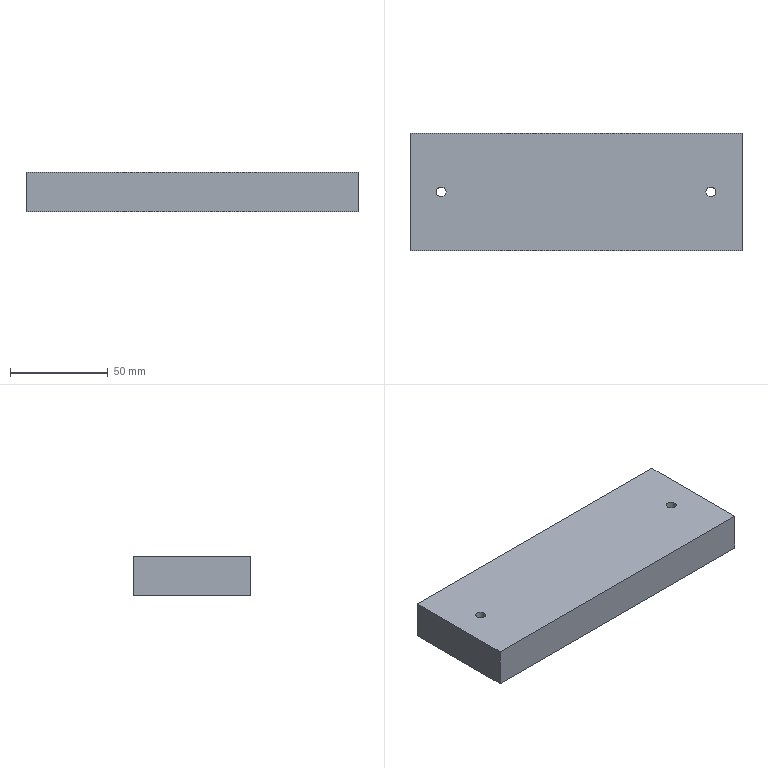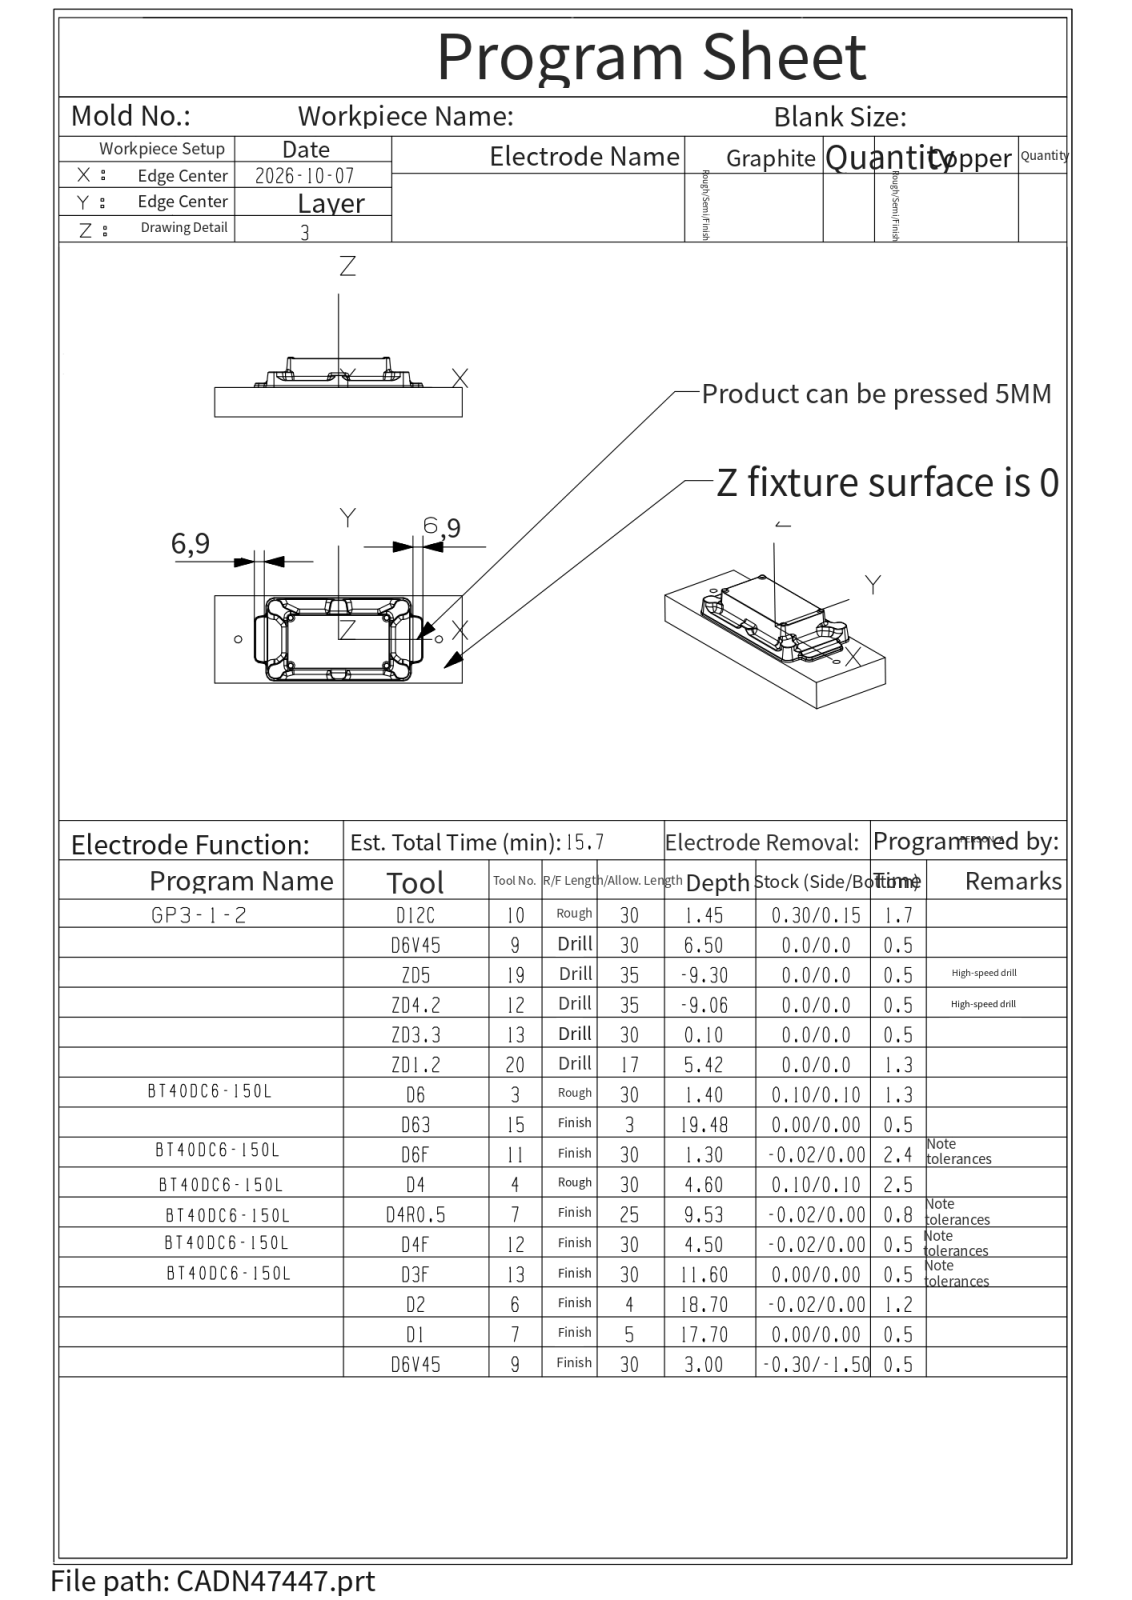NC program | NX | posted by the shop | part box 170 x 60 x 20 mm
Lines 6151 to 7072 of 17682:
T05 M06
T20
( name=D3    T=5 )
( XY = 0.10 )
( Z = 0.10 )
G00 G90 G54 X-19.944 Y-32.3 S10000 M03
G43 Z27.98 H05 M08
Z17.38
G03 X-19.344 Y-32.9 I.6 J0.0 F1600.
G01 X-18.41 F2000.
G03 X-18. Y-32.5 I.01 J.4
G01 Y-31.556
G03 X-18.6 Y-30.956 I-.6 J0.0
G01 X-19.944 Y-32.3 Z17.18 F6000.
G03 X-19.344 Y-32.9 I.6 J0.0 F1600.
G01 X-18.4 F2000.
G03 X-18. Y-32.5 I0.0 J.4
G01 Y-31.556
G03 X-18.6 Y-30.956 I-.6 J0.0
G01 X-19.944 Y-32.3 Z16.98 F6000.
G03 X-19.344 Y-32.9 I.6 J0.0 F1600.
G01 X-18.4 F2000.
G03 X-18. Y-32.5 I0.0 J.4
G01 Y-31.556
G03 X-18.6 Y-30.956 I-.6 J0.0
G01 X-19.944 Y-32.3 Z16.78 F6000.
G03 X-19.344 Y-32.9 I.6 J0.0 F1600.
G01 X-18.4 F2000.
G03 X-18. Y-32.5 I0.0 J.4
G01 Y-31.556
G03 X-18.6 Y-30.956 I-.6 J0.0
G01 X-19.944 Y-32.3 Z16.58 F6000.
G03 X-19.344 Y-32.9 I.6 J0.0 F1600.
G01 X-18.4 F2000.
G03 X-18. Y-32.5 I0.0 J.4
G01 Y-31.556
G03 X-18.6 Y-30.956 I-.6 J0.0
G01 X-19.944 Y-32.3 Z16.38 F6000.
G03 X-19.344 Y-32.9 I.6 J0.0 F1600.
G01 X-18.4 F2000.
G03 X-18. Y-32.5 I0.0 J.4
G01 Y-31.556
G03 X-18.6 Y-30.956 I-.6 J0.0
G01 X-19.944 Y-32.3 Z16.18 F6000.
G03 X-19.344 Y-32.9 I.6 J0.0 F1600.
G01 X-18.4 F2000.
G03 X-18. Y-32.5 I0.0 J.4
G01 Y-31.556
G03 X-18.6 Y-30.956 I-.6 J0.0
G01 X-19.944 Y-32.3 Z15.98 F6000.
G03 X-19.344 Y-32.9 I.6 J0.0 F1600.
G01 X-18.4 F2000.
G03 X-18. Y-32.5 I0.0 J.4
G01 Y-31.556
G03 X-18.6 Y-30.956 I-.6 J0.0
G01 X-19.944 Y-32.3 Z15.78 F6000.
G03 X-19.344 Y-32.9 I.6 J0.0 F1600.
G01 X-18.4 F2000.
G03 X-18. Y-32.5 I0.0 J.4
G01 Y-31.556
G03 X-18.6 Y-30.956 I-.6 J0.0
G01 X-19.944 Y-32.3 Z15.58 F6000.
G03 X-19.344 Y-32.9 I.6 J0.0 F1600.
G01 X-18.4 F2000.
G03 X-18. Y-32.5 I0.0 J.4
G01 Y-31.556
G03 X-18.6 Y-30.956 I-.6 J0.0
G01 X-19.944 Y-32.3 Z15.38 F6000.
G03 X-19.344 Y-32.9 I.6 J0.0 F1600.
G01 X-18.4 F2000.
G03 X-18. Y-32.5 I0.0 J.4
G01 Y-31.556
G03 X-18.6 Y-30.956 I-.6 J0.0
G01 X-19.944 Y-32.3 Z15.18 F6000.
G03 X-19.344 Y-32.9 I.6 J0.0 F1600.
G01 X-18.4 F2000.
G03 X-18. Y-32.5 I0.0 J.4
G01 Y-31.556
G03 X-18.6 Y-30.956 I-.6 J0.0
G01 X-19.944 Y-32.3 Z14.98 F6000.
G03 X-19.344 Y-32.9 I.6 J0.0 F1600.
G01 X-18.4 F2000.
G03 X-18. Y-32.5 I0.0 J.4
G01 Y-31.556
G03 X-18.6 Y-30.956 I-.6 J0.0
G01 X-19.944 Y-32.3 Z14.78 F6000.
G03 X-19.344 Y-32.9 I.6 J0.0 F1600.
G01 X-18.4 F2000.
G03 X-18. Y-32.5 I0.0 J.4
G01 Y-31.556
G03 X-18.6 Y-30.956 I-.6 J0.0
G01 X-19.944 Y-32.3 Z14.58 F6000.
G03 X-19.344 Y-32.9 I.6 J0.0 F1600.
G01 X-18.4 F2000.
G03 X-18. Y-32.5 I0.0 J.4
G01 Y-31.556
G03 X-18.6 Y-30.956 I-.6 J0.0
G01 X-19.944 Y-32.3 Z14.38 F6000.
G03 X-19.344 Y-32.9 I.6 J0.0 F1600.
G01 X-18.4 F2000.
G03 X-18. Y-32.5 I0.0 J.4
G01 Y-31.556
G03 X-18.6 Y-30.956 I-.6 J0.0
G01 X-19.944 Y-32.3 Z14.18 F6000.
G03 X-19.344 Y-32.9 I.6 J0.0 F1600.
G01 X-18.4 F2000.
G03 X-18. Y-32.5 I0.0 J.4
G01 Y-31.556
G03 X-18.6 Y-30.956 I-.6 J0.0
G01 X-19.944 Y-32.3 Z13.98 F6000.
G03 X-19.344 Y-32.9 I.6 J0.0 F1600.
G01 X-18.4 F2000.
G03 X-18. Y-32.5 I0.0 J.4
G01 Y-31.556
G03 X-18.6 Y-30.956 I-.6 J0.0
G01 X-19.944 Y-32.3 Z13.78 F6000.
G03 X-19.344 Y-32.9 I.6 J0.0 F1600.
G01 X-18.4 F2000.
G03 X-18. Y-32.5 I0.0 J.4
G01 Y-31.556
G03 X-18.6 Y-30.956 I-.6 J0.0
G01 X-19.944 Y-32.3 Z13.58 F6000.
G03 X-19.344 Y-32.9 I.6 J0.0 F1600.
G01 X-18.4 F2000.
G03 X-18. Y-32.5 I0.0 J.4
G01 Y-31.556
G03 X-18.6 Y-30.956 I-.6 J0.0
G01 X-19.944 Y-32.3 Z13.38 F6000.
G03 X-19.344 Y-32.9 I.6 J0.0 F1600.
G01 X-18.4 F2000.
G03 X-18. Y-32.5 I0.0 J.4
G01 Y-31.556
G03 X-18.6 Y-30.956 I-.6 J0.0
G01 X-19.944 Y-32.3 Z13.18 F6000.
G03 X-19.344 Y-32.9 I.6 J0.0 F1600.
G01 X-18.4 F2000.
G03 X-18. Y-32.5 I0.0 J.4
G01 Y-31.556
G03 X-18.6 Y-30.956 I-.6 J0.0
G01 X-19.944 Y-32.3 Z12.98 F6000.
G03 X-19.344 Y-32.9 I.6 J0.0 F1600.
G01 X-18.4 F2000.
G03 X-18. Y-32.5 I0.0 J.4
G01 Y-31.556
G03 X-18.6 Y-30.956 I-.6 J0.0
G01 X-19.944 Y-32.3 Z12.78 F6000.
G03 X-19.344 Y-32.9 I.6 J0.0 F1600.
G01 X-18.4 F2000.
G03 X-18. Y-32.5 I0.0 J.4
G01 Y-31.556
G03 X-18.6 Y-30.956 I-.6 J0.0
G01 X-19.944 Y-32.3 Z12.58 F6000.
G03 X-19.344 Y-32.9 I.6 J0.0 F1600.
G01 X-18.4 F2000.
G03 X-18. Y-32.5 I0.0 J.4
G01 Y-31.556
G03 X-18.6 Y-30.956 I-.6 J0.0
G01 X-19.944 Y-32.3 Z12.38 F6000.
G03 X-19.344 Y-32.9 I.6 J0.0 F1600.
G01 X-18.4 F2000.
G03 X-18. Y-32.5 I0.0 J.4
G01 Y-31.556
G03 X-18.6 Y-30.956 I-.6 J0.0
G01 X-19.944 Y-32.3 Z12.18 F6000.
G03 X-19.344 Y-32.9 I.6 J0.0 F1600.
G01 X-18.4 F2000.
G03 X-18. Y-32.5 I0.0 J.4
G01 Y-31.556
G03 X-18.6 Y-30.956 I-.6 J0.0
G01 X-19.944 Y-32.3 Z11.98 F6000.
G03 X-19.344 Y-32.9 I.6 J0.0 F1600.
G01 X-18.4 F2000.
G03 X-18. Y-32.5 I0.0 J.4
G01 Y-31.556
G03 X-18.6 Y-30.956 I-.6 J0.0
G01 X-19.944 Y-32.3 Z11.78 F6000.
G03 X-19.344 Y-32.9 I.6 J0.0 F1600.
G01 X-18.4 F2000.
G03 X-18. Y-32.5 I0.0 J.4
G01 Y-31.556
G03 X-18.6 Y-30.956 I-.6 J0.0
G01 X-19.944 Y-32.3 Z11.58 F6000.
G03 X-19.344 Y-32.9 I.6 J0.0 F1600.
G01 X-18.4 F2000.
G03 X-18. Y-32.5 I0.0 J.4
G01 Y-31.556
G03 X-18.6 Y-30.956 I-.6 J0.0
G01 X-19.944 Y-32.3 Z11.38 F6000.
G03 X-19.344 Y-32.9 I.6 J0.0 F1600.
G01 X-18.4 F2000.
G03 X-18. Y-32.5 I0.0 J.4
G01 Y-31.556
G03 X-18.6 Y-30.956 I-.6 J0.0
G01 X-19.944 Y-32.3 Z11.18 F6000.
G03 X-19.344 Y-32.9 I.6 J0.0 F1600.
G01 X-18.4 F2000.
G03 X-18. Y-32.5 I0.0 J.4
G01 Y-31.556
G03 X-18.6 Y-30.956 I-.6 J0.0
G01 X-19.944 Y-32.3 Z10.98 F6000.
G03 X-19.344 Y-32.9 I.6 J0.0 F1600.
G01 X-18.4 F2000.
G03 X-18. Y-32.5 I0.0 J.4
G01 Y-31.556
G03 X-18.6 Y-30.956 I-.6 J0.0
G01 X-19.944 Y-32.3 Z10.78 F6000.
G03 X-19.344 Y-32.9 I.6 J0.0 F1600.
G01 X-18.4 F2000.
G03 X-18. Y-32.5 I0.0 J.4
G01 Y-31.556
G03 X-18.6 Y-30.956 I-.6 J0.0
G01 X-19.944 Y-32.3 Z10.58 F6000.
G03 X-19.344 Y-32.9 I.6 J0.0 F1600.
G01 X-18.4 F2000.
G03 X-18. Y-32.5 I0.0 J.4
G01 Y-31.556
G03 X-18.6 Y-30.956 I-.6 J0.0
G01 X-19.944 Y-32.3 Z10.38 F6000.
G03 X-19.344 Y-32.9 I.6 J0.0 F1600.
G01 X-18.4 F2000.
G03 X-18. Y-32.5 I0.0 J.4
G01 Y-31.556
G03 X-18.6 Y-30.956 I-.6 J0.0
G01 X-19.944 Y-32.3 Z10.18 F6000.
G03 X-19.344 Y-32.9 I.6 J0.0 F1600.
G01 X-18.4 F2000.
G03 X-18. Y-32.5 I0.0 J.4
G01 Y-31.556
G03 X-18.6 Y-30.956 I-.6 J0.0
G01 X-19.944 Y-32.3 Z9.98 F6000.
G03 X-19.344 Y-32.9 I.6 J0.0 F1600.
G01 X-18.4 F2000.
G03 X-18. Y-32.5 I0.0 J.4
G01 Y-31.556
G03 X-18.6 Y-30.956 I-.6 J0.0
G01 X-19.944 Y-32.3 Z9.78 F6000.
G03 X-19.344 Y-32.9 I.6 J0.0 F1600.
G01 X-18.4 F2000.
G03 X-18. Y-32.5 I0.0 J.4
G01 Y-31.556
G03 X-18.6 Y-30.956 I-.6 J0.0
G01 X-19.944 Y-32.3 Z9.58 F6000.
G03 X-19.344 Y-32.9 I.6 J0.0 F1600.
G01 X-18.4 F2000.
G03 X-18. Y-32.5 I0.0 J.4
G01 Y-31.556
G03 X-18.6 Y-30.956 I-.6 J0.0
G01 X-19.944 Y-32.3 Z9.38 F6000.
G03 X-19.344 Y-32.9 I.6 J0.0 F1600.
G01 X-18.4 F2000.
G03 X-18. Y-32.5 I0.0 J.4
G01 Y-31.556
G03 X-18.6 Y-30.956 I-.6 J0.0
G01 X-19.944 Y-32.3 Z9.18 F6000.
G03 X-19.344 Y-32.9 I.6 J0.0 F1600.
G01 X-18.4 F2000.
G03 X-18. Y-32.5 I0.0 J.4
G01 Y-31.556
G03 X-18.6 Y-30.956 I-.6 J0.0
G01 X-19.944 Y-32.3 Z8.98 F6000.
G03 X-19.344 Y-32.9 I.6 J0.0 F1600.
G01 X-18.4 F2000.
G03 X-18. Y-32.5 I0.0 J.4
G01 Y-31.556
G03 X-18.6 Y-30.956 I-.6 J0.0
G01 X-19.944 Y-32.3 Z8.78 F6000.
G03 X-19.344 Y-32.9 I.6 J0.0 F1600.
G01 X-18.4 F2000.
G03 X-18. Y-32.5 I0.0 J.4
G01 Y-31.556
G03 X-18.6 Y-30.956 I-.6 J0.0
G01 X-19.944 Y-32.3 Z8.58 F6000.
G03 X-19.344 Y-32.9 I.6 J0.0 F1600.
G01 X-18.4 F2000.
G03 X-18. Y-32.5 I0.0 J.4
G01 Y-31.556
G03 X-18.6 Y-30.956 I-.6 J0.0
G01 X-19.944 Y-32.3 Z8.38 F6000.
G03 X-19.344 Y-32.9 I.6 J0.0 F1600.
G01 X-18.4 F2000.
G03 X-18. Y-32.5 I0.0 J.4
G01 Y-31.556
G03 X-18.6 Y-30.956 I-.6 J0.0
G01 X-19.944 Y-32.3 Z8.18 F6000.
G03 X-19.344 Y-32.9 I.6 J0.0 F1600.
G01 X-18.4 F2000.
G03 X-18. Y-32.5 I0.0 J.4
G01 Y-31.556
G03 X-18.6 Y-30.956 I-.6 J0.0
G01 X-19.944 Y-32.3 Z7.98 F6000.
G03 X-19.344 Y-32.9 I.6 J0.0 F1600.
G01 X-18.4 F2000.
G03 X-18. Y-32.5 I0.0 J.4
G01 Y-31.556
G03 X-18.6 Y-30.956 I-.6 J0.0
G01 X-19.944 Y-32.3 Z7.78 F6000.
G03 X-19.344 Y-32.9 I.6 J0.0 F1600.
G01 X-18.4 F2000.
G03 X-18. Y-32.5 I0.0 J.4
G01 Y-31.556
G03 X-18.6 Y-30.956 I-.6 J0.0
G01 X-19.944 Y-32.3 Z7.58 F6000.
G03 X-19.344 Y-32.9 I.6 J0.0 F1600.
G01 X-18.4 F2000.
G03 X-18. Y-32.5 I0.0 J.4
G01 Y-31.556
G03 X-18.6 Y-30.956 I-.6 J0.0
G01 X-19.944 Y-32.3 Z7.38 F6000.
G03 X-19.344 Y-32.9 I.6 J0.0 F1600.
G01 X-18.4 F2000.
G03 X-18. Y-32.5 I0.0 J.4
G01 Y-31.556
G03 X-18.6 Y-30.956 I-.6 J0.0
G01 X-19.944 Y-32.3 Z7.18 F6000.
G03 X-19.344 Y-32.9 I.6 J0.0 F1600.
G01 X-18.4 F2000.
G03 X-18. Y-32.5 I0.0 J.4
G01 Y-31.556
G03 X-18.6 Y-30.956 I-.6 J0.0
G01 X-19.944 Y-32.3 Z6.98 F6000.
G03 X-19.344 Y-32.9 I.6 J0.0 F1600.
G01 X-18.4 F2000.
G03 X-18. Y-32.5 I0.0 J.4
G01 Y-31.556
G03 X-18.6 Y-30.956 I-.6 J0.0
G01 X-19.944 Y-32.3 Z6.78 F6000.
G03 X-19.344 Y-32.9 I.6 J0.0 F1600.
G01 X-18.4 F2000.
G03 X-18. Y-32.5 I0.0 J.4
G01 Y-31.556
G03 X-18.6 Y-30.956 I-.6 J0.0
G01 X-19.944 Y-32.3 Z6.58 F6000.
G03 X-19.344 Y-32.9 I.6 J0.0 F1600.
G01 X-18.4 F2000.
G03 X-18. Y-32.5 I0.0 J.4
G01 Y-31.556
G03 X-18.6 Y-30.956 I-.6 J0.0
G01 X-19.944 Y-32.3 Z6.38 F6000.
G03 X-19.344 Y-32.9 I.6 J0.0 F1600.
G01 X-18.4 F2000.
G03 X-18. Y-32.5 I0.0 J.4
G01 Y-31.556
G03 X-18.6 Y-30.956 I-.6 J0.0
G01 X-19.944 Y-32.3 Z6.18 F6000.
G03 X-19.344 Y-32.9 I.6 J0.0 F1600.
G01 X-18.4 F2000.
G03 X-18. Y-32.5 I0.0 J.4
G01 Y-31.556
G03 X-18.6 Y-30.956 I-.6 J0.0
G01 X-19.944 Y-32.3 Z5.98 F6000.
G03 X-19.344 Y-32.9 I.6 J0.0 F1600.
G01 X-18.4 F2000.
G03 X-18. Y-32.5 I0.0 J.4
G01 Y-31.556
G03 X-18.6 Y-30.956 I-.6 J0.0
G01 X-19.944 Y-32.3 Z5.78 F6000.
G03 X-19.344 Y-32.9 I.6 J0.0 F1600.
G01 X-18.4 F2000.
G03 X-18. Y-32.5 I0.0 J.4
G01 Y-31.556
G03 X-18.6 Y-30.956 I-.6 J0.0
G01 X-19.944 Y-32.3 Z5.58 F6000.
G03 X-19.344 Y-32.9 I.6 J0.0 F1600.
G01 X-18.4 F2000.
G03 X-18. Y-32.5 I0.0 J.4
G01 Y-31.556
G03 X-18.6 Y-30.956 I-.6 J0.0
G01 X-19.944 Y-32.3 Z5.38 F6000.
G03 X-19.344 Y-32.9 I.6 J0.0 F1600.
G01 X-18.4 F2000.
G03 X-18. Y-32.5 I0.0 J.4
G01 Y-31.556
G03 X-18.6 Y-30.956 I-.6 J0.0
G01 X-19.944 Y-32.3 Z5.18 F6000.
G03 X-19.344 Y-32.9 I.6 J0.0 F1600.
G01 X-18.4 F2000.
G03 X-18. Y-32.5 I0.0 J.4
G01 Y-31.556
G03 X-18.6 Y-30.956 I-.6 J0.0
G01 X-19.944 Y-32.3 Z4.98 F6000.
G03 X-19.344 Y-32.9 I.6 J0.0 F1600.
G01 X-18.4 F2000.
G03 X-18. Y-32.5 I0.0 J.4
G01 Y-31.556
G03 X-18.6 Y-30.956 I-.6 J0.0
G01 X-19.944 Y-32.3 Z4.78 F6000.
G03 X-19.344 Y-32.9 I.6 J0.0 F1600.
G01 X-18.4 F2000.
G03 X-18. Y-32.5 I0.0 J.4
G01 Y-31.556
G03 X-18.6 Y-30.956 I-.6 J0.0
G01 X-19.944 Y-32.3 Z4.58 F6000.
G03 X-19.344 Y-32.9 I.6 J0.0 F1600.
G01 X-18.4 F2000.
G03 X-18. Y-32.5 I0.0 J.4
G01 Y-31.556
G03 X-18.6 Y-30.956 I-.6 J0.0
G01 X-19.944 Y-32.3 Z4.38 F6000.
G03 X-19.344 Y-32.9 I.6 J0.0 F1600.
G01 X-18.4 F2000.
G03 X-18. Y-32.5 I0.0 J.4
G01 Y-31.556
G03 X-18.6 Y-30.956 I-.6 J0.0
G01 X-19.944 Y-32.3 Z4.18 F6000.
G03 X-19.344 Y-32.9 I.6 J0.0 F1600.
G01 X-18.4 F2000.
G03 X-18. Y-32.5 I0.0 J.4
G01 Y-31.556
G03 X-18.6 Y-30.956 I-.6 J0.0
G01 X-19.944 Y-32.3 Z3.98 F6000.
G03 X-19.344 Y-32.9 I.6 J0.0 F1600.
G01 X-18.4 F2000.
G03 X-18. Y-32.5 I0.0 J.4
G01 Y-31.556
G03 X-18.6 Y-30.956 I-.6 J0.0
G01 X-19.944 Y-32.3 Z3.78 F6000.
G03 X-19.344 Y-32.9 I.6 J0.0 F1600.
G01 X-18.4 F2000.
G03 X-18. Y-32.5 I0.0 J.4
G01 Y-31.556
G03 X-18.6 Y-30.956 I-.6 J0.0
G01 X-19.944 Y-32.3 Z3.58 F6000.
G03 X-19.344 Y-32.9 I.6 J0.0 F1600.
G01 X-18.4 F2000.
G03 X-18. Y-32.5 I0.0 J.4
G01 Y-31.556
G03 X-18.6 Y-30.956 I-.6 J0.0
G00 Z27.98
Y-25.044
Z17.38
G03 X-18. Y-24.444 I0.0 J.6 F1600.
G01 Y-23.5 F2000.
G03 X-18.4 Y-23.1 I-.4 J0.0
G01 X-19.344
G03 X-19.944 Y-23.7 I0.0 J-.6
G01 X-18.6 Y-25.044 Z17.18 F6000.
G03 X-18. Y-24.444 I0.0 J.6 F1600.
G01 Y-23.5 F2000.
G03 X-18.4 Y-23.1 I-.4 J0.0
G01 X-19.344
G03 X-19.944 Y-23.7 I0.0 J-.6
G01 X-18.6 Y-25.044 Z16.98 F6000.
G03 X-18. Y-24.444 I0.0 J.6 F1600.
G01 Y-23.5 F2000.
G03 X-18.4 Y-23.1 I-.4 J0.0
G01 X-19.344
G03 X-19.944 Y-23.7 I0.0 J-.6
G01 X-18.6 Y-25.044 Z16.78 F6000.
G03 X-18. Y-24.444 I0.0 J.6 F1600.
G01 Y-23.5 F2000.
G03 X-18.4 Y-23.1 I-.4 J0.0
G01 X-19.344
G03 X-19.944 Y-23.7 I0.0 J-.6
G01 X-18.6 Y-25.044 Z16.58 F6000.
G03 X-18. Y-24.444 I0.0 J.6 F1600.
G01 Y-23.5 F2000.
G03 X-18.4 Y-23.1 I-.4 J0.0
G01 X-19.344
G03 X-19.944 Y-23.7 I0.0 J-.6
G01 X-18.6 Y-25.044 Z16.38 F6000.
G03 X-18. Y-24.444 I0.0 J.6 F1600.
G01 Y-23.5 F2000.
G03 X-18.4 Y-23.1 I-.4 J0.0
G01 X-19.344
G03 X-19.944 Y-23.7 I0.0 J-.6
G01 X-18.6 Y-25.044 Z16.18 F6000.
G03 X-18. Y-24.444 I0.0 J.6 F1600.
G01 Y-23.5 F2000.
G03 X-18.4 Y-23.1 I-.4 J0.0
G01 X-19.344
G03 X-19.944 Y-23.7 I0.0 J-.6
G01 X-18.6 Y-25.044 Z15.98 F6000.
G03 X-18. Y-24.444 I0.0 J.6 F1600.
G01 Y-23.5 F2000.
G03 X-18.4 Y-23.1 I-.4 J0.0
G01 X-19.344
G03 X-19.944 Y-23.7 I0.0 J-.6
G01 X-18.6 Y-25.044 Z15.78 F6000.
G03 X-18. Y-24.444 I0.0 J.6 F1600.
G01 Y-23.5 F2000.
G03 X-18.4 Y-23.1 I-.4 J0.0
G01 X-19.344
G03 X-19.944 Y-23.7 I0.0 J-.6
G01 X-18.6 Y-25.044 Z15.58 F6000.
G03 X-18. Y-24.444 I0.0 J.6 F1600.
G01 Y-23.5 F2000.
G03 X-18.4 Y-23.1 I-.4 J0.0
G01 X-19.344
G03 X-19.944 Y-23.7 I0.0 J-.6
G01 X-18.6 Y-25.044 Z15.38 F6000.
G03 X-18. Y-24.444 I0.0 J.6 F1600.
G01 Y-23.5 F2000.
G03 X-18.4 Y-23.1 I-.4 J0.0
G01 X-19.344
G03 X-19.944 Y-23.7 I0.0 J-.6
G01 X-18.6 Y-25.044 Z15.18 F6000.
G03 X-18. Y-24.444 I0.0 J.6 F1600.
G01 Y-23.5 F2000.
G03 X-18.4 Y-23.1 I-.4 J0.0
G01 X-19.344
G03 X-19.944 Y-23.7 I0.0 J-.6
G01 X-18.6 Y-25.044 Z14.98 F6000.
G03 X-18. Y-24.444 I0.0 J.6 F1600.
G01 Y-23.5 F2000.
G03 X-18.4 Y-23.1 I-.4 J0.0
G01 X-19.344
G03 X-19.944 Y-23.7 I0.0 J-.6
G01 X-18.6 Y-25.044 Z14.78 F6000.
G03 X-18. Y-24.444 I0.0 J.6 F1600.
G01 Y-23.5 F2000.
G03 X-18.4 Y-23.1 I-.4 J0.0
G01 X-19.344
G03 X-19.944 Y-23.7 I0.0 J-.6
G01 X-18.6 Y-25.044 Z14.58 F6000.
G03 X-18. Y-24.444 I0.0 J.6 F1600.
G01 Y-23.5 F2000.
G03 X-18.4 Y-23.1 I-.4 J0.0
G01 X-19.344
G03 X-19.944 Y-23.7 I0.0 J-.6
G01 X-18.6 Y-25.044 Z14.38 F6000.
G03 X-18. Y-24.444 I0.0 J.6 F1600.
G01 Y-23.5 F2000.
G03 X-18.4 Y-23.1 I-.4 J0.0
G01 X-19.344
G03 X-19.944 Y-23.7 I0.0 J-.6
G01 X-18.6 Y-25.044 Z14.18 F6000.
G03 X-18. Y-24.444 I0.0 J.6 F1600.
G01 Y-23.5 F2000.
G03 X-18.4 Y-23.1 I-.4 J0.0
G01 X-19.344
G03 X-19.944 Y-23.7 I0.0 J-.6
G01 X-18.6 Y-25.044 Z13.98 F6000.
G03 X-18. Y-24.444 I0.0 J.6 F1600.
G01 Y-23.5 F2000.
G03 X-18.4 Y-23.1 I-.4 J0.0
G01 X-19.344
G03 X-19.944 Y-23.7 I0.0 J-.6
G01 X-18.6 Y-25.044 Z13.78 F6000.
G03 X-18. Y-24.444 I0.0 J.6 F1600.
G01 Y-23.5 F2000.
G03 X-18.4 Y-23.1 I-.4 J0.0
G01 X-19.344
G03 X-19.944 Y-23.7 I0.0 J-.6
G01 X-18.6 Y-25.044 Z13.58 F6000.
G03 X-18. Y-24.444 I0.0 J.6 F1600.
G01 Y-23.5 F2000.
G03 X-18.4 Y-23.1 I-.4 J0.0
G01 X-19.344
G03 X-19.944 Y-23.7 I0.0 J-.6
G01 X-18.6 Y-25.044 Z13.38 F6000.
G03 X-18. Y-24.444 I0.0 J.6 F1600.
G01 Y-23.5 F2000.
G03 X-18.4 Y-23.1 I-.4 J0.0
G01 X-19.344
G03 X-19.944 Y-23.7 I0.0 J-.6
G01 X-18.6 Y-25.044 Z13.18 F6000.
G03 X-18. Y-24.444 I0.0 J.6 F1600.
G01 Y-23.5 F2000.
G03 X-18.4 Y-23.1 I-.4 J0.0
G01 X-19.344
G03 X-19.944 Y-23.7 I0.0 J-.6
G01 X-18.6 Y-25.044 Z12.98 F6000.
G03 X-18. Y-24.444 I0.0 J.6 F1600.
G01 Y-23.5 F2000.
G03 X-18.4 Y-23.1 I-.4 J0.0
G01 X-19.344
G03 X-19.944 Y-23.7 I0.0 J-.6
G01 X-18.6 Y-25.044 Z12.78 F6000.
G03 X-18. Y-24.444 I0.0 J.6 F1600.
G01 Y-23.5 F2000.
G03 X-18.4 Y-23.1 I-.4 J0.0
G01 X-19.344
G03 X-19.944 Y-23.7 I0.0 J-.6
G01 X-18.6 Y-25.044 Z12.58 F6000.
G03 X-18. Y-24.444 I0.0 J.6 F1600.
G01 Y-23.5 F2000.
G03 X-18.4 Y-23.1 I-.4 J0.0
G01 X-19.344
G03 X-19.944 Y-23.7 I0.0 J-.6
G01 X-18.6 Y-25.044 Z12.38 F6000.
G03 X-18. Y-24.444 I0.0 J.6 F1600.
G01 Y-23.5 F2000.
G03 X-18.4 Y-23.1 I-.4 J0.0
G01 X-19.344
G03 X-19.944 Y-23.7 I0.0 J-.6
G01 X-18.6 Y-25.044 Z12.18 F6000.
G03 X-18. Y-24.444 I0.0 J.6 F1600.
G01 Y-23.5 F2000.
G03 X-18.4 Y-23.1 I-.4 J0.0
G01 X-19.344
G03 X-19.944 Y-23.7 I0.0 J-.6
G01 X-18.6 Y-25.044 Z11.98 F6000.
G03 X-18. Y-24.444 I0.0 J.6 F1600.
G01 Y-23.5 F2000.
G03 X-18.4 Y-23.1 I-.4 J0.0
G01 X-19.344
G03 X-19.944 Y-23.7 I0.0 J-.6
G01 X-18.6 Y-25.044 Z11.78 F6000.
G03 X-18. Y-24.444 I0.0 J.6 F1600.
G01 Y-23.5 F2000.
G03 X-18.4 Y-23.1 I-.4 J0.0
G01 X-19.344
G03 X-19.944 Y-23.7 I0.0 J-.6
G01 X-18.6 Y-25.044 Z11.58 F6000.
G03 X-18. Y-24.444 I0.0 J.6 F1600.
G01 Y-23.5 F2000.
G03 X-18.4 Y-23.1 I-.4 J0.0
G01 X-19.344
G03 X-19.944 Y-23.7 I0.0 J-.6
G01 X-18.6 Y-25.044 Z11.38 F6000.
G03 X-18. Y-24.444 I0.0 J.6 F1600.
G01 Y-23.5 F2000.
G03 X-18.4 Y-23.1 I-.4 J0.0
G01 X-19.344
G03 X-19.944 Y-23.7 I0.0 J-.6
G01 X-18.6 Y-25.044 Z11.18 F6000.
G03 X-18. Y-24.444 I0.0 J.6 F1600.
G01 Y-23.5 F2000.
G03 X-18.4 Y-23.1 I-.4 J0.0
G01 X-19.344
G03 X-19.944 Y-23.7 I0.0 J-.6
G01 X-18.6 Y-25.044 Z10.98 F6000.
G03 X-18. Y-24.444 I0.0 J.6 F1600.
G01 Y-23.5 F2000.
G03 X-18.4 Y-23.1 I-.4 J0.0
G01 X-19.344
G03 X-19.944 Y-23.7 I0.0 J-.6
G01 X-18.6 Y-25.044 Z10.78 F6000.
G03 X-18. Y-24.444 I0.0 J.6 F1600.
G01 Y-23.5 F2000.
G03 X-18.4 Y-23.1 I-.4 J0.0
G01 X-19.344
G03 X-19.944 Y-23.7 I0.0 J-.6
G01 X-18.6 Y-25.044 Z10.58 F6000.
G03 X-18. Y-24.444 I0.0 J.6 F1600.
G01 Y-23.5 F2000.
G03 X-18.4 Y-23.1 I-.4 J0.0
G01 X-19.344
G03 X-19.944 Y-23.7 I0.0 J-.6
G01 X-18.6 Y-25.044 Z10.38 F6000.
G03 X-18. Y-24.444 I0.0 J.6 F1600.
G01 Y-23.5 F2000.
G03 X-18.4 Y-23.1 I-.4 J0.0
G01 X-19.344
G03 X-19.944 Y-23.7 I0.0 J-.6
G01 X-18.6 Y-25.044 Z10.18 F6000.
G03 X-18. Y-24.444 I0.0 J.6 F1600.
G01 Y-23.5 F2000.
G03 X-18.4 Y-23.1 I-.4 J0.0
G01 X-19.344
G03 X-19.944 Y-23.7 I0.0 J-.6
G01 X-18.6 Y-25.044 Z9.98 F6000.
G03 X-18. Y-24.444 I0.0 J.6 F1600.
G01 Y-23.5 F2000.
G03 X-18.4 Y-23.1 I-.4 J0.0
G01 X-19.344
G03 X-19.944 Y-23.7 I0.0 J-.6
G01 X-18.6 Y-25.044 Z9.78 F6000.
G03 X-18. Y-24.444 I0.0 J.6 F1600.
G01 Y-23.5 F2000.
G03 X-18.4 Y-23.1 I-.4 J0.0
G01 X-19.344
G03 X-19.944 Y-23.7 I0.0 J-.6
G01 X-18.6 Y-25.044 Z9.58 F6000.
G03 X-18. Y-24.444 I0.0 J.6 F1600.
G01 Y-23.5 F2000.
G03 X-18.4 Y-23.1 I-.4 J0.0
G01 X-19.344
G03 X-19.944 Y-23.7 I0.0 J-.6
G01 X-18.6 Y-25.044 Z9.38 F6000.
G03 X-18. Y-24.444 I0.0 J.6 F1600.
G01 Y-23.5 F2000.
G03 X-18.4 Y-23.1 I-.4 J0.0
G01 X-19.344
G03 X-19.944 Y-23.7 I0.0 J-.6
G01 X-18.6 Y-25.044 Z9.18 F6000.
G03 X-18. Y-24.444 I0.0 J.6 F1600.
G01 Y-23.5 F2000.
G03 X-18.4 Y-23.1 I-.4 J0.0
G01 X-19.344
G03 X-19.944 Y-23.7 I0.0 J-.6
G01 X-18.6 Y-25.044 Z8.98 F6000.
G03 X-18. Y-24.444 I0.0 J.6 F1600.
G01 Y-23.5 F2000.
G03 X-18.4 Y-23.1 I-.4 J0.0
G01 X-19.344
G03 X-19.944 Y-23.7 I0.0 J-.6
G01 X-18.6 Y-25.044 Z8.78 F6000.
G03 X-18. Y-24.444 I0.0 J.6 F1600.
G01 Y-23.5 F2000.
G03 X-18.4 Y-23.1 I-.4 J0.0
G01 X-19.344
G03 X-19.944 Y-23.7 I0.0 J-.6
G01 X-18.6 Y-25.044 Z8.58 F6000.
G03 X-18. Y-24.444 I0.0 J.6 F1600.
G01 Y-23.5 F2000.
G03 X-18.4 Y-23.1 I-.4 J0.0
G01 X-19.344
G03 X-19.944 Y-23.7 I0.0 J-.6
G01 X-18.6 Y-25.044 Z8.38 F6000.
G03 X-18. Y-24.444 I0.0 J.6 F1600.
G01 Y-23.5 F2000.
G03 X-18.4 Y-23.1 I-.4 J0.0
G01 X-19.344
G03 X-19.944 Y-23.7 I0.0 J-.6
G01 X-18.6 Y-25.044 Z8.18 F6000.
G03 X-18. Y-24.444 I0.0 J.6 F1600.
G01 Y-23.5 F2000.
G03 X-18.4 Y-23.1 I-.4 J0.0
G01 X-19.344
G03 X-19.944 Y-23.7 I0.0 J-.6
G01 X-18.6 Y-25.044 Z7.98 F6000.
G03 X-18. Y-24.444 I0.0 J.6 F1600.
G01 Y-23.5 F2000.
G03 X-18.4 Y-23.1 I-.4 J0.0
G01 X-19.344
G03 X-19.944 Y-23.7 I0.0 J-.6
G01 X-18.6 Y-25.044 Z7.78 F6000.
G03 X-18. Y-24.444 I0.0 J.6 F1600.
G01 Y-23.5 F2000.
G03 X-18.4 Y-23.1 I-.4 J0.0
G01 X-19.344
G03 X-19.944 Y-23.7 I0.0 J-.6
G01 X-18.6 Y-25.044 Z7.58 F6000.
G03 X-18. Y-24.444 I0.0 J.6 F1600.
G01 Y-23.5 F2000.
G03 X-18.4 Y-23.1 I-.4 J0.0
G01 X-19.344
G03 X-19.944 Y-23.7 I0.0 J-.6
G01 X-18.6 Y-25.044 Z7.38 F6000.
G03 X-18. Y-24.444 I0.0 J.6 F1600.
G01 Y-23.5 F2000.
G03 X-18.4 Y-23.1 I-.4 J0.0
G01 X-19.344
G03 X-19.944 Y-23.7 I0.0 J-.6
G01 X-18.6 Y-25.044 Z7.18 F6000.
G03 X-18. Y-24.444 I0.0 J.6 F1600.
G01 Y-23.5 F2000.
G03 X-18.4 Y-23.1 I-.4 J0.0
G01 X-19.344
G03 X-19.944 Y-23.7 I0.0 J-.6
G01 X-18.6 Y-25.044 Z6.98 F6000.
G03 X-18. Y-24.444 I0.0 J.6 F1600.
G01 Y-23.5 F2000.
G03 X-18.4 Y-23.1 I-.4 J0.0
G01 X-19.344
G03 X-19.944 Y-23.7 I0.0 J-.6
G01 X-18.6 Y-25.044 Z6.78 F6000.
G03 X-18. Y-24.444 I0.0 J.6 F1600.
G01 Y-23.5 F2000.
G03 X-18.4 Y-23.1 I-.4 J0.0
G01 X-19.344
G03 X-19.944 Y-23.7 I0.0 J-.6
G01 X-18.6 Y-25.044 Z6.58 F6000.
G03 X-18. Y-24.444 I0.0 J.6 F1600.
G01 Y-23.5 F2000.
G03 X-18.4 Y-23.1 I-.4 J0.0
G01 X-19.344
G03 X-19.944 Y-23.7 I0.0 J-.6
G01 X-18.6 Y-25.044 Z6.38 F6000.
G03 X-18. Y-24.444 I0.0 J.6 F1600.
G01 Y-23.5 F2000.
G03 X-18.4 Y-23.1 I-.4 J0.0
G01 X-19.344
G03 X-19.944 Y-23.7 I0.0 J-.6
G01 X-18.6 Y-25.044 Z6.18 F6000.
G03 X-18. Y-24.444 I0.0 J.6 F1600.
G01 Y-23.5 F2000.
G03 X-18.4 Y-23.1 I-.4 J0.0
G01 X-19.344
G03 X-19.944 Y-23.7 I0.0 J-.6
G01 X-18.6 Y-25.044 Z5.98 F6000.
G03 X-18. Y-24.444 I0.0 J.6 F1600.
G01 Y-23.5 F2000.
G03 X-18.4 Y-23.1 I-.4 J0.0
G01 X-19.344
G03 X-19.944 Y-23.7 I0.0 J-.6
G01 X-18.6 Y-25.044 Z5.78 F6000.
G03 X-18. Y-24.444 I0.0 J.6 F1600.
G01 Y-23.5 F2000.
G03 X-18.4 Y-23.1 I-.4 J0.0
G01 X-19.344
G03 X-19.944 Y-23.7 I0.0 J-.6
G01 X-18.6 Y-25.044 Z5.58 F6000.
G03 X-18. Y-24.444 I0.0 J.6 F1600.
G01 Y-23.5 F2000.
G03 X-18.4 Y-23.1 I-.4 J0.0
G01 X-19.344
G03 X-19.944 Y-23.7 I0.0 J-.6
G01 X-18.6 Y-25.044 Z5.38 F6000.
G03 X-18. Y-24.444 I0.0 J.6 F1600.
G01 Y-23.5 F2000.
G03 X-18.4 Y-23.1 I-.4 J0.0
G01 X-19.344
G03 X-19.944 Y-23.7 I0.0 J-.6
G01 X-18.6 Y-25.044 Z5.18 F6000.
G03 X-18. Y-24.444 I0.0 J.6 F1600.
G01 Y-23.5 F2000.
G03 X-18.4 Y-23.1 I-.4 J0.0
G01 X-19.344
G03 X-19.944 Y-23.7 I0.0 J-.6
G01 X-18.6 Y-25.044 Z4.98 F6000.
G03 X-18. Y-24.444 I0.0 J.6 F1600.
G01 Y-23.5 F2000.
G03 X-18.4 Y-23.1 I-.4 J0.0
G01 X-19.344
G03 X-19.944 Y-23.7 I0.0 J-.6
G01 X-18.6 Y-25.044 Z4.78 F6000.
G03 X-18. Y-24.444 I0.0 J.6 F1600.
G01 Y-23.5 F2000.
G03 X-18.4 Y-23.1 I-.4 J0.0
G01 X-19.344
G03 X-19.944 Y-23.7 I0.0 J-.6
G01 X-18.6 Y-25.044 Z4.58 F6000.
G03 X-18. Y-24.444 I0.0 J.6 F1600.
G01 Y-23.5 F2000.
G03 X-18.4 Y-23.1 I-.4 J0.0
G01 X-19.344
G03 X-19.944 Y-23.7 I0.0 J-.6
G01 X-18.6 Y-25.044 Z4.38 F6000.
G03 X-18. Y-24.444 I0.0 J.6 F1600.
G01 Y-23.5 F2000.
G03 X-18.4 Y-23.1 I-.4 J0.0
G01 X-19.344
G03 X-19.944 Y-23.7 I0.0 J-.6
G01 X-18.6 Y-25.044 Z4.18 F6000.
G03 X-18. Y-24.444 I0.0 J.6 F1600.
G01 Y-23.5 F2000.
G03 X-18.4 Y-23.1 I-.4 J0.0
G01 X-19.344
G03 X-19.944 Y-23.7 I0.0 J-.6
G01 X-18.6 Y-25.044 Z3.98 F6000.
G03 X-18. Y-24.444 I0.0 J.6 F1600.
G01 Y-23.5 F2000.
G03 X-18.4 Y-23.1 I-.4 J0.0
G01 X-19.344
G03 X-19.944 Y-23.7 I0.0 J-.6
G01 X-18.6 Y-25.044 Z3.78 F6000.
G03 X-18. Y-24.444 I0.0 J.6 F1600.
G01 Y-23.5 F2000.
G03 X-18.4 Y-23.1 I-.4 J0.0
G01 X-19.344
G03 X-19.944 Y-23.7 I0.0 J-.6
G01 X-18.6 Y-25.044 Z3.58 F6000.
G03 X-18. Y-24.444 I0.0 J.6 F1600.
G01 Y-23.5 F2000.
G03 X-18.4 Y-23.1 I-.4 J0.0
G01 X-19.344
G03 X-19.944 Y-23.7 I0.0 J-.6
G00 Z27.98
X-46.616 Y-22.202
Z17.38
G03 X-46.458 Y-21.399 I-.352 J.486 F1600.
G02 X-47. Y-19.5 I3.058 J1.899 F2000.
G01 Y-17.01
G03 X-47.8 Y-17. I-.4 J.01
G01 Y-21.627
G03 X-47.2 Y-22.227 I.6 J0.0
G01 X-46.617 Y-22.2 Z17.18 F6000.
G03 X-46.459 Y-21.397 I-.352 J.486 F1600.
G02 X-47. Y-19.5 I3.059 J1.897 F2000.
G01 Y-17.
G03 X-47.8 I-.4 J0.0
G01 Y-21.622
G03 X-47.2 Y-22.222 I.6 J0.0
G01 X-46.617 Y-22.2 Z16.98 F6000.
G03 X-46.459 Y-21.397 I-.352 J.486 F1600.
G02 X-47. Y-19.5 I3.059 J1.897 F2000.
G01 Y-17.
G03 X-47.8 I-.4 J0.0
G01 Y-21.622
G03 X-47.2 Y-22.222 I.6 J0.0
G01 X-46.617 Y-22.2 Z16.78 F6000.
G03 X-46.459 Y-21.397 I-.352 J.486 F1600.
G02 X-47. Y-19.5 I3.059 J1.897 F2000.
G01 Y-17.
G03 X-47.8 I-.4 J0.0
G01 Y-21.622
G03 X-47.2 Y-22.222 I.6 J0.0
G01 X-46.617 Y-22.2 Z16.58 F6000.
G03 X-46.459 Y-21.397 I-.352 J.486 F1600.
G02 X-47. Y-19.5 I3.059 J1.897 F2000.
G01 Y-17.
G03 X-47.8 I-.4 J0.0
G01 Y-21.622
G03 X-47.2 Y-22.222 I.6 J0.0
G01 X-46.617 Y-22.2 Z16.38 F6000.
G03 X-46.459 Y-21.397 I-.352 J.486 F1600.
G02 X-47. Y-19.5 I3.059 J1.897 F2000.
G01 Y-17.
G03 X-47.8 I-.4 J0.0
G01 Y-21.622
G03 X-47.2 Y-22.222 I.6 J0.0
G01 X-46.617 Y-22.2 Z16.18 F6000.
G03 X-46.459 Y-21.397 I-.352 J.486 F1600.
G02 X-47. Y-19.5 I3.059 J1.897 F2000.
G01 Y-17.
G03 X-47.8 I-.4 J0.0
G01 Y-21.622
G03 X-47.2 Y-22.222 I.6 J0.0
G01 X-46.617 Y-22.2 Z15.98 F6000.
G03 X-46.459 Y-21.397 I-.352 J.486 F1600.
G02 X-47. Y-19.5 I3.059 J1.897 F2000.
G01 Y-17.
G03 X-47.8 I-.4 J0.0
G01 Y-21.622
G03 X-47.2 Y-22.222 I.6 J0.0
G01 X-46.617 Y-22.2 Z15.78 F6000.
G03 X-46.459 Y-21.397 I-.352 J.486 F1600.
G02 X-47. Y-19.5 I3.059 J1.897 F2000.
G01 Y-17.
G03 X-47.8 I-.4 J0.0
G01 Y-21.622
G03 X-47.2 Y-22.222 I.6 J0.0
G01 X-46.617 Y-22.2 Z15.58 F6000.
G03 X-46.459 Y-21.397 I-.352 J.486 F1600.
G02 X-47. Y-19.5 I3.059 J1.897 F2000.
G01 Y-17.
G03 X-47.8 I-.4 J0.0
G01 Y-21.622
G03 X-47.2 Y-22.222 I.6 J0.0
G01 X-46.617 Y-22.2 Z15.38 F6000.